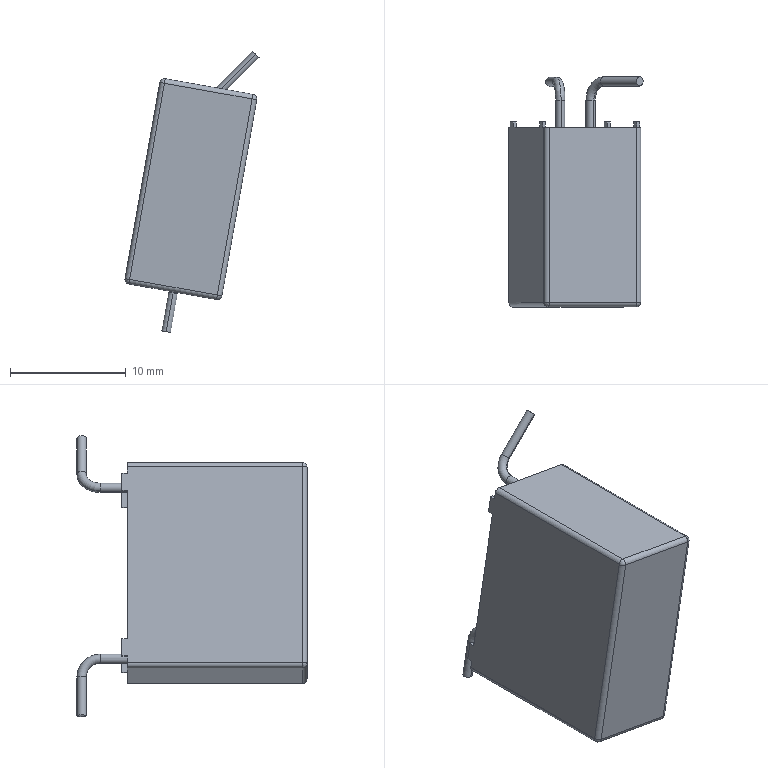Part | SolidWorks | features BaseBody 1 | 1 solid | 557 faces | box 11.583 x 19.87 x 24.283 mm | volume 2380 mm3 | plane 533 | cylinder 16 | sphere 4 | torus 4 | commonest cylinder face diameters 0.8 x16